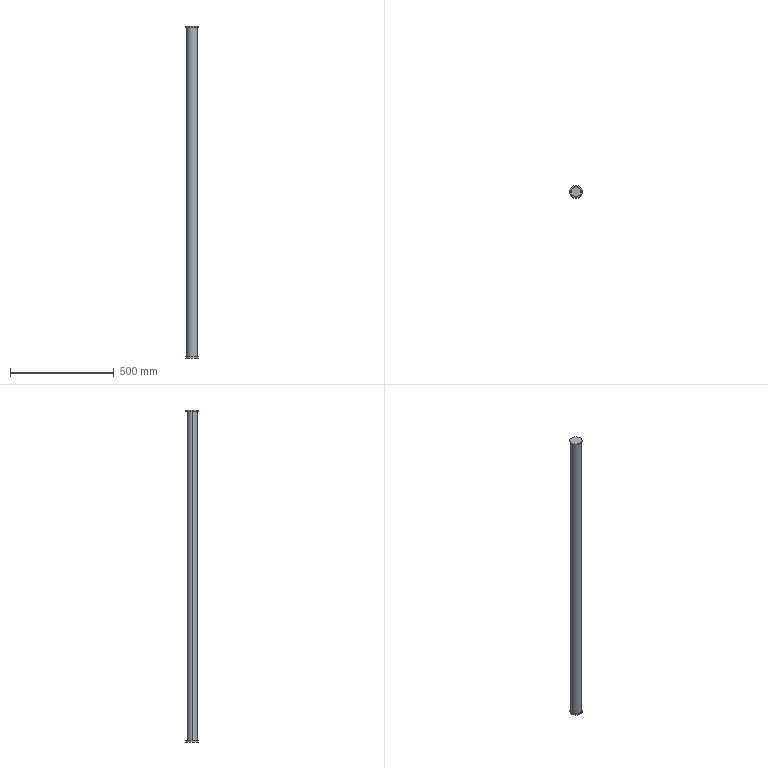Part | SolidWorks | features ICE 2, Extrusion 1, Fillet 1, RefAxis 1, RevCut 1 | 1 solid | 14 faces | box 60 x 60 x 1600 mm | volume 273036 mm3 | cylinder 8 | plane 6 | commonest cylinder face diameters 60 x4 48 x2 50 x2
STEP:
#1=CARTESIAN_POINT('',(30.,0.,1595.));
#2=VERTEX_POINT('',#1);
#3=CARTESIAN_POINT('',(-30.,0.,1595.));
#4=VERTEX_POINT('',#3);
#5=CARTESIAN_POINT('',(0.,0.,1595.));
#6=DIRECTION('',(0.,0.,1.));
#7=DIRECTION('',(1.,0.,0.));
#8=AXIS2_PLACEMENT_3D('',#5,#6,#7);
#9=CIRCLE('',#8,30.);
#10=EDGE_CURVE('',#2,#4,#9,.T.);
#11=ORIENTED_EDGE('',*,*,#10,.F.);
#12=CARTESIAN_POINT('',(30.,0.,1590.));
#13=VERTEX_POINT('',#12);
#14=CARTESIAN_POINT('',(30.,0.,1595.));
#15=DIRECTION('',(0.,0.,-1.));
#16=VECTOR('',#15,1000.);
#17=LINE('',#14,#16);
#18=EDGE_CURVE('',#2,#13,#17,.T.);
#19=ORIENTED_EDGE('',*,*,#18,.T.);
#20=CARTESIAN_POINT('',(-30.,0.,1590.));
#21=VERTEX_POINT('',#20);
#22=CARTESIAN_POINT('',(0.,0.,1590.));
#23=DIRECTION('',(0.,0.,1.));
#24=DIRECTION('',(1.,0.,0.));
#25=AXIS2_PLACEMENT_3D('',#22,#23,#24);
#26=CIRCLE('',#25,30.);
#27=EDGE_CURVE('',#13,#21,#26,.T.);
#28=ORIENTED_EDGE('',*,*,#27,.T.);
#29=CARTESIAN_POINT('',(-30.,0.,1595.));
#30=DIRECTION('',(0.,0.,-1.));
#31=VECTOR('',#30,1000.);
#32=LINE('',#29,#31);
#33=EDGE_CURVE('',#4,#21,#32,.T.);
#34=ORIENTED_EDGE('',*,*,#33,.F.);
#35=EDGE_LOOP('',(#11,#19,#28,#34));
#36=FACE_OUTER_BOUND('',#35,.T.);
#37=CARTESIAN_POINT('',(0.,0.,1595.));
#38=DIRECTION('',(0.,0.,-1.));
#39=DIRECTION('',(-1.,0.,0.));
#40=AXIS2_PLACEMENT_3D('',#37,#38,#39);
#41=CYLINDRICAL_SURFACE('',#40,30.);
#42=ADVANCED_FACE('',(#36),#41,.T.);
#43=CARTESIAN_POINT('',(-30.,0.,-5.));
#44=VERTEX_POINT('',#43);
#45=CARTESIAN_POINT('',(30.,0.,-5.));
#46=VERTEX_POINT('',#45);
#47=CARTESIAN_POINT('',(0.,0.,-5.));
#48=DIRECTION('',(0.,0.,-1.));
#49=DIRECTION('',(-1.,0.,0.));
#50=AXIS2_PLACEMENT_3D('',#47,#48,#49);
#51=CIRCLE('',#50,30.);
#52=EDGE_CURVE('',#44,#46,#51,.T.);
#53=ORIENTED_EDGE('',*,*,#52,.F.);
#54=CARTESIAN_POINT('',(-30.,0.,0.));
#55=VERTEX_POINT('',#54);
#56=CARTESIAN_POINT('',(-30.,0.,-5.));
#57=DIRECTION('',(0.,0.,1.));
#58=VECTOR('',#57,1000.);
#59=LINE('',#56,#58);
#60=EDGE_CURVE('',#44,#55,#59,.T.);
#61=ORIENTED_EDGE('',*,*,#60,.T.);
#62=CARTESIAN_POINT('',(30.,0.,0.));
#63=VERTEX_POINT('',#62);
#64=CARTESIAN_POINT('',(0.,0.,0.));
#65=DIRECTION('',(0.,0.,-1.));
#66=DIRECTION('',(-1.,0.,0.));
#67=AXIS2_PLACEMENT_3D('',#64,#65,#66);
#68=CIRCLE('',#67,30.);
#69=EDGE_CURVE('',#55,#63,#68,.T.);
#70=ORIENTED_EDGE('',*,*,#69,.T.);
#71=CARTESIAN_POINT('',(30.,0.,-5.));
#72=DIRECTION('',(0.,0.,1.));
#73=VECTOR('',#72,1000.);
#74=LINE('',#71,#73);
#75=EDGE_CURVE('',#46,#63,#74,.T.);
#76=ORIENTED_EDGE('',*,*,#75,.F.);
#77=EDGE_LOOP('',(#53,#61,#70,#76));
#78=FACE_OUTER_BOUND('',#77,.T.);
#79=CARTESIAN_POINT('',(0.,0.,-5.));
#80=DIRECTION('',(0.,0.,1.));
#81=DIRECTION('',(1.,0.,0.));
#82=AXIS2_PLACEMENT_3D('',#79,#80,#81);
#83=CYLINDRICAL_SURFACE('',#82,30.);
#84=ADVANCED_FACE('',(#78),#83,.T.);
#85=CARTESIAN_POINT('',(25.,0.,1590.));
#86=VERTEX_POINT('',#85);
#87=CARTESIAN_POINT('',(-25.,0.,1590.));
#88=VERTEX_POINT('',#87);
#89=CARTESIAN_POINT('',(0.,0.,1590.));
#90=DIRECTION('',(0.,0.,1.));
#91=DIRECTION('',(1.,0.,0.));
#92=AXIS2_PLACEMENT_3D('',#89,#90,#91);
#93=CIRCLE('',#92,25.);
#94=EDGE_CURVE('',#86,#88,#93,.T.);
#95=ORIENTED_EDGE('',*,*,#94,.F.);
#96=CARTESIAN_POINT('',(25.,0.,0.));
#97=VERTEX_POINT('',#96);
#98=CARTESIAN_POINT('',(25.,0.,1590.));
#99=DIRECTION('',(0.,0.,-1.));
#100=VECTOR('',#99,1000.);
#101=LINE('',#98,#100);
#102=EDGE_CURVE('',#86,#97,#101,.T.);
#103=ORIENTED_EDGE('',*,*,#102,.T.);
#104=CARTESIAN_POINT('',(-25.,0.,0.));
#105=VERTEX_POINT('',#104);
#106=CARTESIAN_POINT('',(0.,0.,0.));
#107=DIRECTION('',(0.,0.,1.));
#108=DIRECTION('',(1.,0.,0.));
#109=AXIS2_PLACEMENT_3D('',#106,#107,#108);
#110=CIRCLE('',#109,25.);
#111=EDGE_CURVE('',#97,#105,#110,.T.);
#112=ORIENTED_EDGE('',*,*,#111,.T.);
#113=CARTESIAN_POINT('',(-25.,0.,1590.));
#114=DIRECTION('',(0.,0.,-1.));
#115=VECTOR('',#114,1000.);
#116=LINE('',#113,#115);
#117=EDGE_CURVE('',#88,#105,#116,.T.);
#118=ORIENTED_EDGE('',*,*,#117,.F.);
#119=EDGE_LOOP('',(#95,#103,#112,#118));
#120=FACE_OUTER_BOUND('',#119,.T.);
#121=CARTESIAN_POINT('',(0.,0.,1590.));
#122=DIRECTION('',(0.,0.,-1.));
#123=DIRECTION('',(-1.,0.,0.));
#124=AXIS2_PLACEMENT_3D('',#121,#122,#123);
#125=CYLINDRICAL_SURFACE('',#124,25.);
#126=ADVANCED_FACE('',(#120),#125,.T.);
#127=ORIENTED_EDGE('',*,*,#102,.F.);
#128=CARTESIAN_POINT('',(0.,0.,1590.));
#129=DIRECTION('',(0.,0.,1.));
#130=DIRECTION('',(1.,0.,0.));
#131=AXIS2_PLACEMENT_3D('',#128,#129,#130);
#132=CIRCLE('',#131,25.);
#133=EDGE_CURVE('',#88,#86,#132,.T.);
#134=ORIENTED_EDGE('',*,*,#133,.F.);
#135=ORIENTED_EDGE('',*,*,#117,.T.);
#136=CARTESIAN_POINT('',(0.,0.,0.));
#137=DIRECTION('',(0.,0.,1.));
#138=DIRECTION('',(1.,0.,0.));
#139=AXIS2_PLACEMENT_3D('',#136,#137,#138);
#140=CIRCLE('',#139,25.);
#141=EDGE_CURVE('',#105,#97,#140,.T.);
#142=ORIENTED_EDGE('',*,*,#141,.T.);
#143=EDGE_LOOP('',(#127,#134,#135,#142));
#144=FACE_OUTER_BOUND('',#143,.T.);
#145=CARTESIAN_POINT('',(0.,0.,1590.));
#146=DIRECTION('',(0.,0.,-1.));
#147=DIRECTION('',(-1.,0.,0.));
#148=AXIS2_PLACEMENT_3D('',#145,#146,#147);
#149=CYLINDRICAL_SURFACE('',#148,25.);
#150=ADVANCED_FACE('',(#144),#149,.T.);
#151=ORIENTED_EDGE('',*,*,#60,.F.);
#152=CARTESIAN_POINT('',(0.,0.,-5.));
#153=DIRECTION('',(0.,0.,-1.));
#154=DIRECTION('',(-1.,0.,0.));
#155=AXIS2_PLACEMENT_3D('',#152,#153,#154);
#156=CIRCLE('',#155,30.);
#157=EDGE_CURVE('',#46,#44,#156,.T.);
#158=ORIENTED_EDGE('',*,*,#157,.F.);
#159=ORIENTED_EDGE('',*,*,#75,.T.);
#160=CARTESIAN_POINT('',(0.,0.,0.));
#161=DIRECTION('',(0.,0.,-1.));
#162=DIRECTION('',(-1.,0.,0.));
#163=AXIS2_PLACEMENT_3D('',#160,#161,#162);
#164=CIRCLE('',#163,30.);
#165=EDGE_CURVE('',#63,#55,#164,.T.);
#166=ORIENTED_EDGE('',*,*,#165,.T.);
#167=EDGE_LOOP('',(#151,#158,#159,#166));
#168=FACE_OUTER_BOUND('',#167,.T.);
#169=CARTESIAN_POINT('',(0.,0.,-5.));
#170=DIRECTION('',(0.,0.,1.));
#171=DIRECTION('',(1.,0.,0.));
#172=AXIS2_PLACEMENT_3D('',#169,#170,#171);
#173=CYLINDRICAL_SURFACE('',#172,30.);
#174=ADVANCED_FACE('',(#168),#173,.T.);
#175=ORIENTED_EDGE('',*,*,#157,.T.);
#176=ORIENTED_EDGE('',*,*,#52,.T.);
#177=EDGE_LOOP('',(#175,#176));
#178=FACE_OUTER_BOUND('',#177,.T.);
#179=CARTESIAN_POINT('',(0.,0.,-5.));
#180=DIRECTION('',(0.,0.,-1.));
#181=DIRECTION('',(-1.,0.,0.));
#182=AXIS2_PLACEMENT_3D('',#179,#180,#181);
#183=PLANE('',#182);
#184=ADVANCED_FACE('',(#178),#183,.T.);
#185=ORIENTED_EDGE('',*,*,#141,.F.);
#186=ORIENTED_EDGE('',*,*,#111,.F.);
#187=EDGE_LOOP('',(#185,#186));
#188=FACE_BOUND('',#187,.T.);
#189=ORIENTED_EDGE('',*,*,#165,.F.);
#190=ORIENTED_EDGE('',*,*,#69,.F.);
#191=EDGE_LOOP('',(#189,#190));
#192=FACE_OUTER_BOUND('',#191,.T.);
#193=CARTESIAN_POINT('',(0.,0.,0.));
#194=DIRECTION('',(0.,0.,-1.));
#195=DIRECTION('',(-1.,0.,0.));
#196=AXIS2_PLACEMENT_3D('',#193,#194,#195);
#197=PLANE('',#196);
#198=ADVANCED_FACE('',(#188,#192),#197,.F.);
#199=ORIENTED_EDGE('',*,*,#18,.F.);
#200=CARTESIAN_POINT('',(0.,0.,1595.));
#201=DIRECTION('',(0.,0.,1.));
#202=DIRECTION('',(1.,0.,0.));
#203=AXIS2_PLACEMENT_3D('',#200,#201,#202);
#204=CIRCLE('',#203,30.);
#205=EDGE_CURVE('',#4,#2,#204,.T.);
#206=ORIENTED_EDGE('',*,*,#205,.F.);
#207=ORIENTED_EDGE('',*,*,#33,.T.);
#208=CARTESIAN_POINT('',(0.,0.,1590.));
#209=DIRECTION('',(0.,0.,1.));
#210=DIRECTION('',(1.,0.,0.));
#211=AXIS2_PLACEMENT_3D('',#208,#209,#210);
#212=CIRCLE('',#211,30.);
#213=EDGE_CURVE('',#21,#13,#212,.T.);
#214=ORIENTED_EDGE('',*,*,#213,.T.);
#215=EDGE_LOOP('',(#199,#206,#207,#214));
#216=FACE_OUTER_BOUND('',#215,.T.);
#217=CARTESIAN_POINT('',(0.,0.,1595.));
#218=DIRECTION('',(0.,0.,-1.));
#219=DIRECTION('',(-1.,0.,0.));
#220=AXIS2_PLACEMENT_3D('',#217,#218,#219);
#221=CYLINDRICAL_SURFACE('',#220,30.);
#222=ADVANCED_FACE('',(#216),#221,.T.);
#223=ORIENTED_EDGE('',*,*,#205,.T.);
#224=ORIENTED_EDGE('',*,*,#10,.T.);
#225=EDGE_LOOP('',(#223,#224));
#226=FACE_OUTER_BOUND('',#225,.T.);
#227=CARTESIAN_POINT('',(0.,0.,1595.));
#228=DIRECTION('',(0.,0.,1.));
#229=DIRECTION('',(1.,0.,0.));
#230=AXIS2_PLACEMENT_3D('',#227,#228,#229);
#231=PLANE('',#230);
#232=ADVANCED_FACE('',(#226),#231,.T.);
#233=ORIENTED_EDGE('',*,*,#133,.T.);
#234=ORIENTED_EDGE('',*,*,#94,.T.);
#235=EDGE_LOOP('',(#233,#234));
#236=FACE_BOUND('',#235,.T.);
#237=ORIENTED_EDGE('',*,*,#213,.F.);
#238=ORIENTED_EDGE('',*,*,#27,.F.);
#239=EDGE_LOOP('',(#237,#238));
#240=FACE_OUTER_BOUND('',#239,.T.);
#241=CARTESIAN_POINT('',(0.,0.,1590.));
#242=DIRECTION('',(0.,0.,1.));
#243=DIRECTION('',(1.,0.,0.));
#244=AXIS2_PLACEMENT_3D('',#241,#242,#243);
#245=PLANE('',#244);
#246=ADVANCED_FACE('',(#236,#240),#245,.F.);
#247=CLOSED_SHELL('',(#42,#84,#126,#150,#174,#184,#198,#222,#232,#246));
#248=CARTESIAN_POINT('',(-24.,0.,1590.));
#249=VERTEX_POINT('',#248);
#250=CARTESIAN_POINT('',(24.,0.,1590.));
#251=VERTEX_POINT('',#250);
#252=CARTESIAN_POINT('',(0.,0.,1590.));
#253=DIRECTION('',(0.,0.,1.));
#254=DIRECTION('',(1.,0.,0.));
#255=AXIS2_PLACEMENT_3D('',#252,#253,#254);
#256=CIRCLE('',#255,24.);
#257=EDGE_CURVE('',#249,#251,#256,.T.);
#258=ORIENTED_EDGE('',*,*,#257,.T.);
#259=CARTESIAN_POINT('',(24.,0.,0.));
#260=VERTEX_POINT('',#259);
#261=CARTESIAN_POINT('',(24.,0.,1590.));
#262=DIRECTION('',(0.,0.,-1.));
#263=VECTOR('',#262,1000.);
#264=LINE('',#261,#263);
#265=EDGE_CURVE('',#251,#260,#264,.T.);
#266=ORIENTED_EDGE('',*,*,#265,.T.);
#267=CARTESIAN_POINT('',(-24.,0.,0.));
#268=VERTEX_POINT('',#267);
#269=CARTESIAN_POINT('',(0.,0.,0.));
#270=DIRECTION('',(0.,0.,1.));
#271=DIRECTION('',(1.,0.,0.));
#272=AXIS2_PLACEMENT_3D('',#269,#270,#271);
#273=CIRCLE('',#272,24.);
#274=EDGE_CURVE('',#268,#260,#273,.T.);
#275=ORIENTED_EDGE('',*,*,#274,.F.);
#276=CARTESIAN_POINT('',(-24.,0.,1590.));
#277=DIRECTION('',(0.,0.,-1.));
#278=VECTOR('',#277,1000.);
#279=LINE('',#276,#278);
#280=EDGE_CURVE('',#249,#268,#279,.T.);
#281=ORIENTED_EDGE('',*,*,#280,.F.);
#282=EDGE_LOOP('',(#258,#266,#275,#281));
#283=FACE_OUTER_BOUND('',#282,.T.);
#284=CARTESIAN_POINT('',(0.,0.,1590.));
#285=DIRECTION('',(0.,0.,-1.));
#286=DIRECTION('',(-1.,0.,0.));
#287=AXIS2_PLACEMENT_3D('',#284,#285,#286);
#288=CYLINDRICAL_SURFACE('',#287,24.);
#289=ADVANCED_FACE('',(#283),#288,.F.);
#290=ORIENTED_EDGE('',*,*,#274,.T.);
#291=CARTESIAN_POINT('',(0.,0.,0.));
#292=DIRECTION('',(0.,0.,1.));
#293=DIRECTION('',(1.,0.,0.));
#294=AXIS2_PLACEMENT_3D('',#291,#292,#293);
#295=CIRCLE('',#294,24.);
#296=EDGE_CURVE('',#260,#268,#295,.T.);
#297=ORIENTED_EDGE('',*,*,#296,.T.);
#298=EDGE_LOOP('',(#290,#297));
#299=FACE_OUTER_BOUND('',#298,.T.);
#300=CARTESIAN_POINT('',(0.,0.,0.));
#301=DIRECTION('',(0.,0.,-1.));
#302=DIRECTION('',(-1.,0.,0.));
#303=AXIS2_PLACEMENT_3D('',#300,#301,#302);
#304=PLANE('',#303);
#305=ADVANCED_FACE('',(#299),#304,.F.);
#306=ORIENTED_EDGE('',*,*,#265,.F.);
#307=CARTESIAN_POINT('',(0.,0.,1590.));
#308=DIRECTION('',(0.,0.,1.));
#309=DIRECTION('',(1.,0.,0.));
#310=AXIS2_PLACEMENT_3D('',#307,#308,#309);
#311=CIRCLE('',#310,24.);
#312=EDGE_CURVE('',#251,#249,#311,.T.);
#313=ORIENTED_EDGE('',*,*,#312,.T.);
#314=ORIENTED_EDGE('',*,*,#280,.T.);
#315=ORIENTED_EDGE('',*,*,#296,.F.);
#316=EDGE_LOOP('',(#306,#313,#314,#315));
#317=FACE_OUTER_BOUND('',#316,.T.);
#318=CARTESIAN_POINT('',(0.,0.,1590.));
#319=DIRECTION('',(0.,0.,-1.));
#320=DIRECTION('',(-1.,0.,0.));
#321=AXIS2_PLACEMENT_3D('',#318,#319,#320);
#322=CYLINDRICAL_SURFACE('',#321,24.);
#323=ADVANCED_FACE('',(#317),#322,.F.);
#324=ORIENTED_EDGE('',*,*,#257,.F.);
#325=ORIENTED_EDGE('',*,*,#312,.F.);
#326=EDGE_LOOP('',(#324,#325));
#327=FACE_OUTER_BOUND('',#326,.T.);
#328=CARTESIAN_POINT('',(0.,0.,1590.));
#329=DIRECTION('',(0.,0.,1.));
#330=DIRECTION('',(1.,0.,0.));
#331=AXIS2_PLACEMENT_3D('',#328,#329,#330);
#332=PLANE('',#331);
#333=ADVANCED_FACE('',(#327),#332,.F.);
#334=CLOSED_SHELL('',(#289,#305,#323,#333));
#335=ORIENTED_CLOSED_SHELL('',*,#334,.F.);
#336=BREP_WITH_VOIDS('',#247,(#335));
#337=CARTESIAN_POINT('',(0.,0.,0.));
#338=DIRECTION('',(0.,0.,1.));
#339=DIRECTION('',(1.,0.,0.));
#340=AXIS2_PLACEMENT_3D('',#337,#338,#339);
#341=(LENGTH_UNIT()NAMED_UNIT(*)SI_UNIT(.MILLI.,.METRE.));
#342=UNCERTAINTY_MEASURE_WITH_UNIT(LENGTH_MEASURE(0.00001),#341,'','');
#343=(NAMED_UNIT(*)PLANE_ANGLE_UNIT()SI_UNIT($,.RADIAN.));
#344=(NAMED_UNIT(*)SI_UNIT($,.STERADIAN.)SOLID_ANGLE_UNIT());
#345=(GEOMETRIC_REPRESENTATION_CONTEXT(3)GLOBAL_UNCERTAINTY_ASSIGNED_CONTEXT((#342))GLOBAL_UNIT_ASSIGNED_CONTEXT((#341,#343,#344))REPRESENTATION_CONTEXT('',''));
#346=ADVANCED_BREP_SHAPE_REPRESENTATION('',(#336,#340),#345);